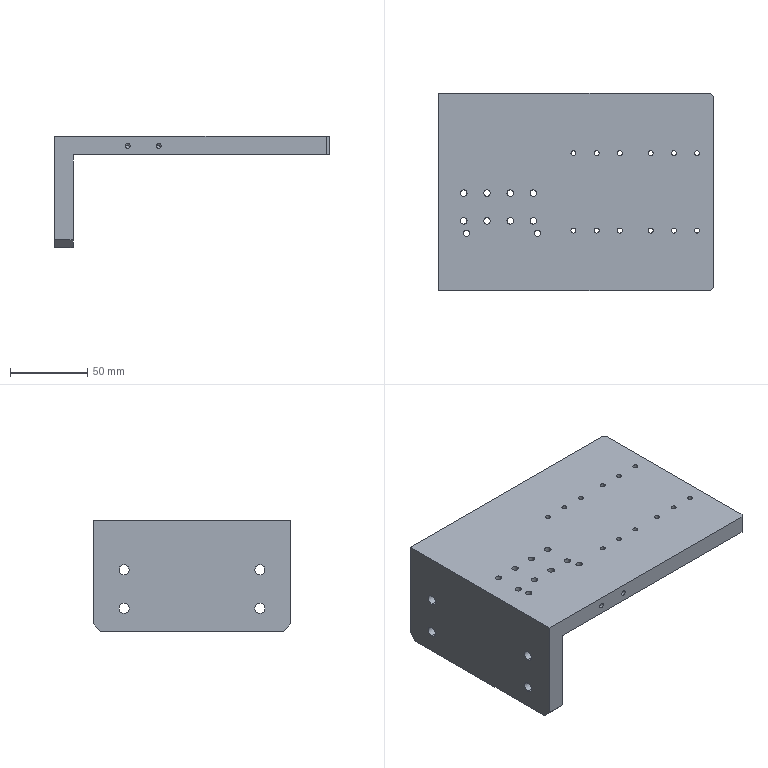Part | STEP file | ASND-0110-Body 1-20 | 1 solid | 80 faces | box 178 x 128 x 72 mm | volume 360301 mm3 | cylinder 60 | plane 12 | cone 8 | commonest cylinder face diameters 3.242 x32 4.2 x16 6.5 x8 4 x4